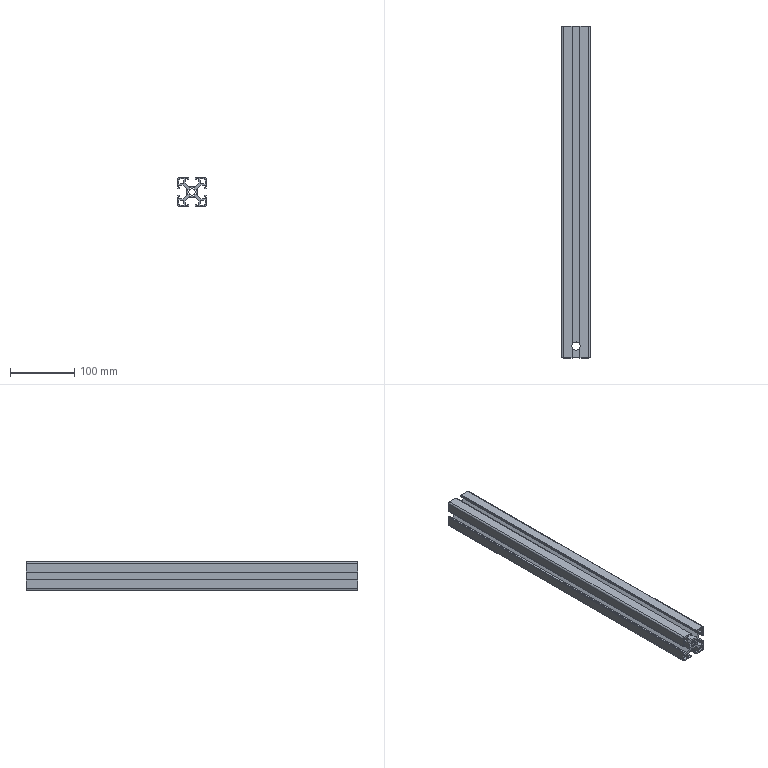Part | STEP file | 1 solid | 188 faces | box 45 x 517 x 45 mm | volume 356541 mm3 | plane 150 | cylinder 38 | commonest cylinder face diameters 10 x18 13 x8 3 x4 5 x4 19 x4